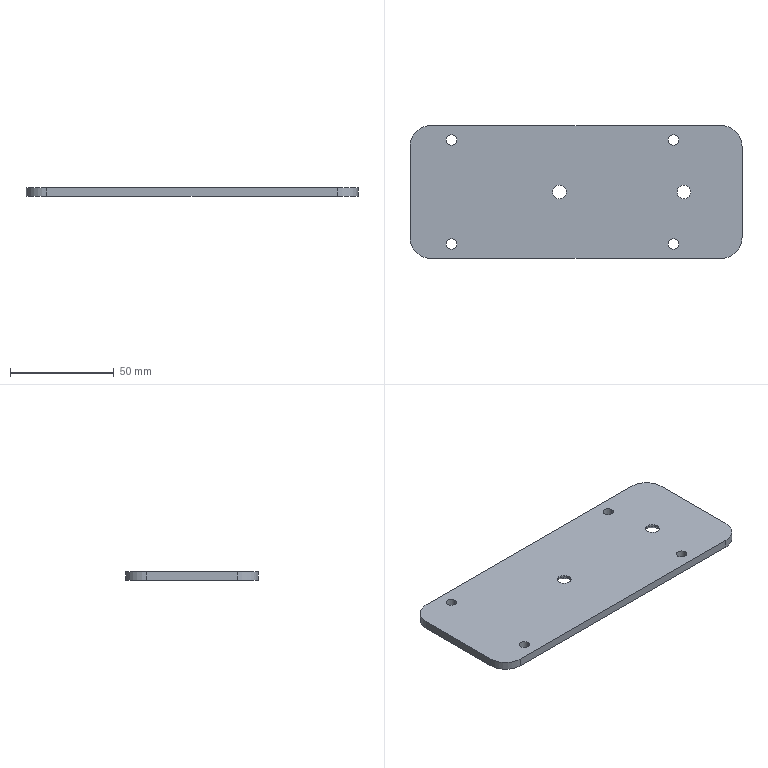Part | SolidWorks | features HoleWzd 2, Extrusion 1, Fillet 1 | 1 solid | 26 faces | box 160 x 64 x 4 mm | volume 39767 mm3 | cylinder 16 | plane 6 | cone 4 | commonest cylinder face diameters 5 x8 6.6 x4 20 x4
STEP:
#1=CARTESIAN_POINT('',(55.3,0.,3.1));
#2=VERTEX_POINT('',#1);
#3=CARTESIAN_POINT('',(48.7,0.,3.1));
#4=VERTEX_POINT('',#3);
#5=CARTESIAN_POINT('',(52.,0.,3.1));
#6=DIRECTION('',(0.,0.,-1.));
#7=DIRECTION('',(-1.,0.,0.));
#8=AXIS2_PLACEMENT_3D('',#5,#6,#7);
#9=CIRCLE('',#8,3.3);
#10=EDGE_CURVE('',#2,#4,#9,.T.);
#11=ORIENTED_EDGE('',*,*,#10,.F.);
#12=CARTESIAN_POINT('',(58.4,0.,0.));
#13=VERTEX_POINT('',#12);
#14=CARTESIAN_POINT('',(58.4,0.,0.));
#15=DIRECTION('',(0.7071,0.,-0.7071));
#16=VECTOR('',#15,1000.);
#17=LINE('',#14,#16);
#18=EDGE_CURVE('',#2,#13,#17,.T.);
#19=ORIENTED_EDGE('',*,*,#18,.T.);
#20=CARTESIAN_POINT('',(45.6,0.,0.));
#21=VERTEX_POINT('',#20);
#22=CARTESIAN_POINT('',(52.,0.,0.));
#23=DIRECTION('',(0.,0.,-1.));
#24=DIRECTION('',(-1.,0.,0.));
#25=AXIS2_PLACEMENT_3D('',#22,#23,#24);
#26=CIRCLE('',#25,6.4);
#27=EDGE_CURVE('',#13,#21,#26,.T.);
#28=ORIENTED_EDGE('',*,*,#27,.T.);
#29=CARTESIAN_POINT('',(45.6,0.,0.));
#30=DIRECTION('',(-0.7071,0.,-0.7071));
#31=VECTOR('',#30,1000.);
#32=LINE('',#29,#31);
#33=EDGE_CURVE('',#4,#21,#32,.T.);
#34=ORIENTED_EDGE('',*,*,#33,.F.);
#35=EDGE_LOOP('',(#11,#19,#28,#34));
#36=FACE_OUTER_BOUND('',#35,.T.);
#37=CARTESIAN_POINT('',(52.,0.,0.));
#38=DIRECTION('',(0.,0.,-1.));
#39=DIRECTION('',(-1.,0.,0.));
#40=AXIS2_PLACEMENT_3D('',#37,#38,#39);
#41=CONICAL_SURFACE('',#40,6.4,0.7854);
#42=ADVANCED_FACE('',(#36),#41,.F.);
#43=CARTESIAN_POINT('',(55.3,0.,4.));
#44=VERTEX_POINT('',#43);
#45=CARTESIAN_POINT('',(48.7,0.,4.));
#46=VERTEX_POINT('',#45);
#47=CARTESIAN_POINT('',(52.,0.,4.));
#48=DIRECTION('',(0.,0.,-1.));
#49=DIRECTION('',(-1.,0.,0.));
#50=AXIS2_PLACEMENT_3D('',#47,#48,#49);
#51=CIRCLE('',#50,3.3);
#52=EDGE_CURVE('',#44,#46,#51,.T.);
#53=ORIENTED_EDGE('',*,*,#52,.F.);
#54=CARTESIAN_POINT('',(55.3,0.,0.));
#55=DIRECTION('',(0.,0.,-1.));
#56=VECTOR('',#55,1000.);
#57=LINE('',#54,#56);
#58=EDGE_CURVE('',#44,#2,#57,.T.);
#59=ORIENTED_EDGE('',*,*,#58,.T.);
#60=ORIENTED_EDGE('',*,*,#10,.T.);
#61=CARTESIAN_POINT('',(48.7,0.,0.));
#62=DIRECTION('',(0.,0.,-1.));
#63=VECTOR('',#62,1000.);
#64=LINE('',#61,#63);
#65=EDGE_CURVE('',#46,#4,#64,.T.);
#66=ORIENTED_EDGE('',*,*,#65,.F.);
#67=EDGE_LOOP('',(#53,#59,#60,#66));
#68=FACE_OUTER_BOUND('',#67,.T.);
#69=CARTESIAN_POINT('',(52.,0.,0.));
#70=DIRECTION('',(0.,0.,-1.));
#71=DIRECTION('',(-1.,0.,0.));
#72=AXIS2_PLACEMENT_3D('',#69,#70,#71);
#73=CYLINDRICAL_SURFACE('',#72,3.3);
#74=ADVANCED_FACE('',(#68),#73,.F.);
#75=CARTESIAN_POINT('',(-4.7,0.,3.1));
#76=VERTEX_POINT('',#75);
#77=CARTESIAN_POINT('',(-11.3,0.,3.1));
#78=VERTEX_POINT('',#77);
#79=CARTESIAN_POINT('',(-8.,0.,3.1));
#80=DIRECTION('',(0.,0.,-1.));
#81=DIRECTION('',(-1.,0.,0.));
#82=AXIS2_PLACEMENT_3D('',#79,#80,#81);
#83=CIRCLE('',#82,3.3);
#84=EDGE_CURVE('',#76,#78,#83,.T.);
#85=ORIENTED_EDGE('',*,*,#84,.F.);
#86=CARTESIAN_POINT('',(-1.6,0.,0.));
#87=VERTEX_POINT('',#86);
#88=CARTESIAN_POINT('',(-1.6,0.,0.));
#89=DIRECTION('',(0.7071,0.,-0.7071));
#90=VECTOR('',#89,1000.);
#91=LINE('',#88,#90);
#92=EDGE_CURVE('',#76,#87,#91,.T.);
#93=ORIENTED_EDGE('',*,*,#92,.T.);
#94=CARTESIAN_POINT('',(-14.4,0.,0.));
#95=VERTEX_POINT('',#94);
#96=CARTESIAN_POINT('',(-8.,0.,0.));
#97=DIRECTION('',(0.,0.,-1.));
#98=DIRECTION('',(-1.,0.,0.));
#99=AXIS2_PLACEMENT_3D('',#96,#97,#98);
#100=CIRCLE('',#99,6.4);
#101=EDGE_CURVE('',#87,#95,#100,.T.);
#102=ORIENTED_EDGE('',*,*,#101,.T.);
#103=CARTESIAN_POINT('',(-14.4,0.,0.));
#104=DIRECTION('',(-0.7071,0.,-0.7071));
#105=VECTOR('',#104,1000.);
#106=LINE('',#103,#105);
#107=EDGE_CURVE('',#78,#95,#106,.T.);
#108=ORIENTED_EDGE('',*,*,#107,.F.);
#109=EDGE_LOOP('',(#85,#93,#102,#108));
#110=FACE_OUTER_BOUND('',#109,.T.);
#111=CARTESIAN_POINT('',(-8.,0.,0.));
#112=DIRECTION('',(0.,0.,-1.));
#113=DIRECTION('',(-1.,0.,0.));
#114=AXIS2_PLACEMENT_3D('',#111,#112,#113);
#115=CONICAL_SURFACE('',#114,6.4,0.7854);
#116=ADVANCED_FACE('',(#110),#115,.F.);
#117=CARTESIAN_POINT('',(-4.7,0.,4.));
#118=VERTEX_POINT('',#117);
#119=CARTESIAN_POINT('',(-11.3,0.,4.));
#120=VERTEX_POINT('',#119);
#121=CARTESIAN_POINT('',(-8.,0.,4.));
#122=DIRECTION('',(0.,0.,-1.));
#123=DIRECTION('',(-1.,0.,0.));
#124=AXIS2_PLACEMENT_3D('',#121,#122,#123);
#125=CIRCLE('',#124,3.3);
#126=EDGE_CURVE('',#118,#120,#125,.T.);
#127=ORIENTED_EDGE('',*,*,#126,.F.);
#128=CARTESIAN_POINT('',(-4.7,0.,0.));
#129=DIRECTION('',(0.,0.,-1.));
#130=VECTOR('',#129,1000.);
#131=LINE('',#128,#130);
#132=EDGE_CURVE('',#118,#76,#131,.T.);
#133=ORIENTED_EDGE('',*,*,#132,.T.);
#134=ORIENTED_EDGE('',*,*,#84,.T.);
#135=CARTESIAN_POINT('',(-11.3,0.,0.));
#136=DIRECTION('',(0.,0.,-1.));
#137=VECTOR('',#136,1000.);
#138=LINE('',#135,#137);
#139=EDGE_CURVE('',#120,#78,#138,.T.);
#140=ORIENTED_EDGE('',*,*,#139,.F.);
#141=EDGE_LOOP('',(#127,#133,#134,#140));
#142=FACE_OUTER_BOUND('',#141,.T.);
#143=CARTESIAN_POINT('',(-8.,0.,0.));
#144=DIRECTION('',(0.,0.,-1.));
#145=DIRECTION('',(-1.,0.,0.));
#146=AXIS2_PLACEMENT_3D('',#143,#144,#145);
#147=CYLINDRICAL_SURFACE('',#146,3.3);
#148=ADVANCED_FACE('',(#142),#147,.F.);
#149=CARTESIAN_POINT('',(-62.5,25.,0.));
#150=VERTEX_POINT('',#149);
#151=CARTESIAN_POINT('',(-57.5,25.,0.));
#152=VERTEX_POINT('',#151);
#153=CARTESIAN_POINT('',(-60.,25.,0.));
#154=DIRECTION('',(0.,0.,1.));
#155=DIRECTION('',(1.,0.,0.));
#156=AXIS2_PLACEMENT_3D('',#153,#154,#155);
#157=CIRCLE('',#156,2.5);
#158=EDGE_CURVE('',#150,#152,#157,.T.);
#159=ORIENTED_EDGE('',*,*,#158,.F.);
#160=CARTESIAN_POINT('',(-62.5,25.,4.));
#161=VERTEX_POINT('',#160);
#162=CARTESIAN_POINT('',(-62.5,25.,4.));
#163=DIRECTION('',(0.,0.,1.));
#164=VECTOR('',#163,1000.);
#165=LINE('',#162,#164);
#166=EDGE_CURVE('',#150,#161,#165,.T.);
#167=ORIENTED_EDGE('',*,*,#166,.T.);
#168=CARTESIAN_POINT('',(-57.5,25.,4.));
#169=VERTEX_POINT('',#168);
#170=CARTESIAN_POINT('',(-60.,25.,4.));
#171=DIRECTION('',(0.,0.,1.));
#172=DIRECTION('',(1.,0.,0.));
#173=AXIS2_PLACEMENT_3D('',#170,#171,#172);
#174=CIRCLE('',#173,2.5);
#175=EDGE_CURVE('',#161,#169,#174,.T.);
#176=ORIENTED_EDGE('',*,*,#175,.T.);
#177=CARTESIAN_POINT('',(-57.5,25.,4.));
#178=DIRECTION('',(0.,0.,1.));
#179=VECTOR('',#178,1000.);
#180=LINE('',#177,#179);
#181=EDGE_CURVE('',#152,#169,#180,.T.);
#182=ORIENTED_EDGE('',*,*,#181,.F.);
#183=EDGE_LOOP('',(#159,#167,#176,#182));
#184=FACE_OUTER_BOUND('',#183,.T.);
#185=CARTESIAN_POINT('',(-60.,25.,4.));
#186=DIRECTION('',(0.,0.,1.));
#187=DIRECTION('',(1.,0.,0.));
#188=AXIS2_PLACEMENT_3D('',#185,#186,#187);
#189=CYLINDRICAL_SURFACE('',#188,2.5);
#190=ADVANCED_FACE('',(#184),#189,.F.);
#191=CARTESIAN_POINT('',(-62.5,-25.,0.));
#192=VERTEX_POINT('',#191);
#193=CARTESIAN_POINT('',(-57.5,-25.,0.));
#194=VERTEX_POINT('',#193);
#195=CARTESIAN_POINT('',(-60.,-25.,0.));
#196=DIRECTION('',(0.,0.,1.));
#197=DIRECTION('',(1.,0.,0.));
#198=AXIS2_PLACEMENT_3D('',#195,#196,#197);
#199=CIRCLE('',#198,2.5);
#200=EDGE_CURVE('',#192,#194,#199,.T.);
#201=ORIENTED_EDGE('',*,*,#200,.F.);
#202=CARTESIAN_POINT('',(-62.5,-25.,4.));
#203=VERTEX_POINT('',#202);
#204=CARTESIAN_POINT('',(-62.5,-25.,4.));
#205=DIRECTION('',(0.,0.,1.));
#206=VECTOR('',#205,1000.);
#207=LINE('',#204,#206);
#208=EDGE_CURVE('',#192,#203,#207,.T.);
#209=ORIENTED_EDGE('',*,*,#208,.T.);
#210=CARTESIAN_POINT('',(-57.5,-25.,4.));
#211=VERTEX_POINT('',#210);
#212=CARTESIAN_POINT('',(-60.,-25.,4.));
#213=DIRECTION('',(0.,0.,1.));
#214=DIRECTION('',(1.,0.,0.));
#215=AXIS2_PLACEMENT_3D('',#212,#213,#214);
#216=CIRCLE('',#215,2.5);
#217=EDGE_CURVE('',#203,#211,#216,.T.);
#218=ORIENTED_EDGE('',*,*,#217,.T.);
#219=CARTESIAN_POINT('',(-57.5,-25.,4.));
#220=DIRECTION('',(0.,0.,1.));
#221=VECTOR('',#220,1000.);
#222=LINE('',#219,#221);
#223=EDGE_CURVE('',#194,#211,#222,.T.);
#224=ORIENTED_EDGE('',*,*,#223,.F.);
#225=EDGE_LOOP('',(#201,#209,#218,#224));
#226=FACE_OUTER_BOUND('',#225,.T.);
#227=CARTESIAN_POINT('',(-60.,-25.,4.));
#228=DIRECTION('',(0.,0.,1.));
#229=DIRECTION('',(1.,0.,0.));
#230=AXIS2_PLACEMENT_3D('',#227,#228,#229);
#231=CYLINDRICAL_SURFACE('',#230,2.5);
#232=ADVANCED_FACE('',(#226),#231,.F.);
#233=CARTESIAN_POINT('',(44.5,25.,0.));
#234=VERTEX_POINT('',#233);
#235=CARTESIAN_POINT('',(49.5,25.,0.));
#236=VERTEX_POINT('',#235);
#237=CARTESIAN_POINT('',(47.,25.,0.));
#238=DIRECTION('',(0.,0.,1.));
#239=DIRECTION('',(1.,0.,0.));
#240=AXIS2_PLACEMENT_3D('',#237,#238,#239);
#241=CIRCLE('',#240,2.5);
#242=EDGE_CURVE('',#234,#236,#241,.T.);
#243=ORIENTED_EDGE('',*,*,#242,.F.);
#244=CARTESIAN_POINT('',(44.5,25.,4.));
#245=VERTEX_POINT('',#244);
#246=CARTESIAN_POINT('',(44.5,25.,4.));
#247=DIRECTION('',(0.,0.,1.));
#248=VECTOR('',#247,1000.);
#249=LINE('',#246,#248);
#250=EDGE_CURVE('',#234,#245,#249,.T.);
#251=ORIENTED_EDGE('',*,*,#250,.T.);
#252=CARTESIAN_POINT('',(49.5,25.,4.));
#253=VERTEX_POINT('',#252);
#254=CARTESIAN_POINT('',(47.,25.,4.));
#255=DIRECTION('',(0.,0.,1.));
#256=DIRECTION('',(1.,0.,0.));
#257=AXIS2_PLACEMENT_3D('',#254,#255,#256);
#258=CIRCLE('',#257,2.5);
#259=EDGE_CURVE('',#245,#253,#258,.T.);
#260=ORIENTED_EDGE('',*,*,#259,.T.);
#261=CARTESIAN_POINT('',(49.5,25.,4.));
#262=DIRECTION('',(0.,0.,1.));
#263=VECTOR('',#262,1000.);
#264=LINE('',#261,#263);
#265=EDGE_CURVE('',#236,#253,#264,.T.);
#266=ORIENTED_EDGE('',*,*,#265,.F.);
#267=EDGE_LOOP('',(#243,#251,#260,#266));
#268=FACE_OUTER_BOUND('',#267,.T.);
#269=CARTESIAN_POINT('',(47.,25.,4.));
#270=DIRECTION('',(0.,0.,1.));
#271=DIRECTION('',(1.,0.,0.));
#272=AXIS2_PLACEMENT_3D('',#269,#270,#271);
#273=CYLINDRICAL_SURFACE('',#272,2.5);
#274=ADVANCED_FACE('',(#268),#273,.F.);
#275=CARTESIAN_POINT('',(44.5,-25.,0.));
#276=VERTEX_POINT('',#275);
#277=CARTESIAN_POINT('',(49.5,-25.,0.));
#278=VERTEX_POINT('',#277);
#279=CARTESIAN_POINT('',(47.,-25.,0.));
#280=DIRECTION('',(0.,0.,1.));
#281=DIRECTION('',(1.,0.,0.));
#282=AXIS2_PLACEMENT_3D('',#279,#280,#281);
#283=CIRCLE('',#282,2.5);
#284=EDGE_CURVE('',#276,#278,#283,.T.);
#285=ORIENTED_EDGE('',*,*,#284,.F.);
#286=CARTESIAN_POINT('',(44.5,-25.,4.));
#287=VERTEX_POINT('',#286);
#288=CARTESIAN_POINT('',(44.5,-25.,4.));
#289=DIRECTION('',(0.,0.,1.));
#290=VECTOR('',#289,1000.);
#291=LINE('',#288,#290);
#292=EDGE_CURVE('',#276,#287,#291,.T.);
#293=ORIENTED_EDGE('',*,*,#292,.T.);
#294=CARTESIAN_POINT('',(49.5,-25.,4.));
#295=VERTEX_POINT('',#294);
#296=CARTESIAN_POINT('',(47.,-25.,4.));
#297=DIRECTION('',(0.,0.,1.));
#298=DIRECTION('',(1.,0.,0.));
#299=AXIS2_PLACEMENT_3D('',#296,#297,#298);
#300=CIRCLE('',#299,2.5);
#301=EDGE_CURVE('',#287,#295,#300,.T.);
#302=ORIENTED_EDGE('',*,*,#301,.T.);
#303=CARTESIAN_POINT('',(49.5,-25.,4.));
#304=DIRECTION('',(0.,0.,1.));
#305=VECTOR('',#304,1000.);
#306=LINE('',#303,#305);
#307=EDGE_CURVE('',#278,#295,#306,.T.);
#308=ORIENTED_EDGE('',*,*,#307,.F.);
#309=EDGE_LOOP('',(#285,#293,#302,#308));
#310=FACE_OUTER_BOUND('',#309,.T.);
#311=CARTESIAN_POINT('',(47.,-25.,4.));
#312=DIRECTION('',(0.,0.,1.));
#313=DIRECTION('',(1.,0.,0.));
#314=AXIS2_PLACEMENT_3D('',#311,#312,#313);
#315=CYLINDRICAL_SURFACE('',#314,2.5);
#316=ADVANCED_FACE('',(#310),#315,.F.);
#317=CARTESIAN_POINT('',(80.,-22.,0.));
#318=VERTEX_POINT('',#317);
#319=CARTESIAN_POINT('',(80.,22.,0.));
#320=VERTEX_POINT('',#319);
#321=CARTESIAN_POINT('',(80.,32.,0.));
#322=DIRECTION('',(0.,1.,0.));
#323=VECTOR('',#322,1000.);
#324=LINE('',#321,#323);
#325=EDGE_CURVE('',#318,#320,#324,.T.);
#326=ORIENTED_EDGE('',*,*,#325,.T.);
#327=CARTESIAN_POINT('',(80.,22.,4.));
#328=VERTEX_POINT('',#327);
#329=CARTESIAN_POINT('',(80.,22.,4.));
#330=DIRECTION('',(0.,0.,1.));
#331=VECTOR('',#330,1000.);
#332=LINE('',#329,#331);
#333=EDGE_CURVE('',#320,#328,#332,.T.);
#334=ORIENTED_EDGE('',*,*,#333,.T.);
#335=CARTESIAN_POINT('',(80.,-22.,4.));
#336=VERTEX_POINT('',#335);
#337=CARTESIAN_POINT('',(80.,32.,4.));
#338=DIRECTION('',(0.,1.,0.));
#339=VECTOR('',#338,1000.);
#340=LINE('',#337,#339);
#341=EDGE_CURVE('',#336,#328,#340,.T.);
#342=ORIENTED_EDGE('',*,*,#341,.F.);
#343=CARTESIAN_POINT('',(80.,-22.,4.));
#344=DIRECTION('',(0.,0.,-1.));
#345=VECTOR('',#344,1000.);
#346=LINE('',#343,#345);
#347=EDGE_CURVE('',#336,#318,#346,.T.);
#348=ORIENTED_EDGE('',*,*,#347,.T.);
#349=EDGE_LOOP('',(#326,#334,#342,#348));
#350=FACE_OUTER_BOUND('',#349,.T.);
#351=CARTESIAN_POINT('',(80.,32.,4.));
#352=DIRECTION('',(-1.,0.,0.));
#353=DIRECTION('',(0.,0.,1.));
#354=AXIS2_PLACEMENT_3D('',#351,#352,#353);
#355=PLANE('',#354);
#356=ADVANCED_FACE('',(#350),#355,.F.);
#357=CARTESIAN_POINT('',(70.,32.,4.));
#358=VERTEX_POINT('',#357);
#359=CARTESIAN_POINT('',(-70.,32.,4.));
#360=VERTEX_POINT('',#359);
#361=CARTESIAN_POINT('',(-80.,32.,4.));
#362=DIRECTION('',(-1.,0.,0.));
#363=VECTOR('',#362,1000.);
#364=LINE('',#361,#363);
#365=EDGE_CURVE('',#358,#360,#364,.T.);
#366=ORIENTED_EDGE('',*,*,#365,.F.);
#367=CARTESIAN_POINT('',(70.,32.,0.));
#368=VERTEX_POINT('',#367);
#369=CARTESIAN_POINT('',(70.,32.,4.));
#370=DIRECTION('',(0.,0.,-1.));
#371=VECTOR('',#370,1000.);
#372=LINE('',#369,#371);
#373=EDGE_CURVE('',#358,#368,#372,.T.);
#374=ORIENTED_EDGE('',*,*,#373,.T.);
#375=CARTESIAN_POINT('',(-70.,32.,0.));
#376=VERTEX_POINT('',#375);
#377=CARTESIAN_POINT('',(-80.,32.,0.));
#378=DIRECTION('',(-1.,0.,0.));
#379=VECTOR('',#378,1000.);
#380=LINE('',#377,#379);
#381=EDGE_CURVE('',#368,#376,#380,.T.);
#382=ORIENTED_EDGE('',*,*,#381,.T.);
#383=CARTESIAN_POINT('',(-70.,32.,4.));
#384=DIRECTION('',(0.,0.,1.));
#385=VECTOR('',#384,1000.);
#386=LINE('',#383,#385);
#387=EDGE_CURVE('',#376,#360,#386,.T.);
#388=ORIENTED_EDGE('',*,*,#387,.T.);
#389=EDGE_LOOP('',(#366,#374,#382,#388));
#390=FACE_OUTER_BOUND('',#389,.T.);
#391=CARTESIAN_POINT('',(-80.,32.,4.));
#392=DIRECTION('',(0.,-1.,0.));
#393=DIRECTION('',(0.,0.,-1.));
#394=AXIS2_PLACEMENT_3D('',#391,#392,#393);
#395=PLANE('',#394);
#396=ADVANCED_FACE('',(#390),#395,.F.);
#397=CARTESIAN_POINT('',(-80.,22.,4.));
#398=VERTEX_POINT('',#397);
#399=CARTESIAN_POINT('',(-80.,-22.,4.));
#400=VERTEX_POINT('',#399);
#401=CARTESIAN_POINT('',(-80.,32.,4.));
#402=DIRECTION('',(0.,-1.,0.));
#403=VECTOR('',#402,1000.);
#404=LINE('',#401,#403);
#405=EDGE_CURVE('',#398,#400,#404,.T.);
#406=ORIENTED_EDGE('',*,*,#405,.F.);
#407=CARTESIAN_POINT('',(-80.,22.,0.));
#408=VERTEX_POINT('',#407);
#409=CARTESIAN_POINT('',(-80.,22.,4.));
#410=DIRECTION('',(0.,0.,-1.));
#411=VECTOR('',#410,1000.);
#412=LINE('',#409,#411);
#413=EDGE_CURVE('',#398,#408,#412,.T.);
#414=ORIENTED_EDGE('',*,*,#413,.T.);
#415=CARTESIAN_POINT('',(-80.,-22.,0.));
#416=VERTEX_POINT('',#415);
#417=CARTESIAN_POINT('',(-80.,32.,0.));
#418=DIRECTION('',(0.,-1.,0.));
#419=VECTOR('',#418,1000.);
#420=LINE('',#417,#419);
#421=EDGE_CURVE('',#408,#416,#420,.T.);
#422=ORIENTED_EDGE('',*,*,#421,.T.);
#423=CARTESIAN_POINT('',(-80.,-22.,4.));
#424=DIRECTION('',(0.,0.,1.));
#425=VECTOR('',#424,1000.);
#426=LINE('',#423,#425);
#427=EDGE_CURVE('',#416,#400,#426,.T.);
#428=ORIENTED_EDGE('',*,*,#427,.T.);
#429=EDGE_LOOP('',(#406,#414,#422,#428));
#430=FACE_OUTER_BOUND('',#429,.T.);
#431=CARTESIAN_POINT('',(-80.,32.,4.));
#432=DIRECTION('',(1.,0.,0.));
#433=DIRECTION('',(0.,1.,0.));
#434=AXIS2_PLACEMENT_3D('',#431,#432,#433);
#435=PLANE('',#434);
#436=ADVANCED_FACE('',(#430),#435,.F.);
#437=CARTESIAN_POINT('',(-70.,-32.,0.));
#438=VERTEX_POINT('',#437);
#439=CARTESIAN_POINT('',(70.,-32.,0.));
#440=VERTEX_POINT('',#439);
#441=CARTESIAN_POINT('',(-80.,-32.,0.));
#442=DIRECTION('',(1.,0.,0.));
#443=VECTOR('',#442,1000.);
#444=LINE('',#441,#443);
#445=EDGE_CURVE('',#438,#440,#444,.T.);
#446=ORIENTED_EDGE('',*,*,#445,.T.);
#447=CARTESIAN_POINT('',(70.,-32.,4.));
#448=VERTEX_POINT('',#447);
#449=CARTESIAN_POINT('',(70.,-32.,4.));
#450=DIRECTION('',(0.,0.,1.));
#451=VECTOR('',#450,1000.);
#452=LINE('',#449,#451);
#453=EDGE_CURVE('',#440,#448,#452,.T.);
#454=ORIENTED_EDGE('',*,*,#453,.T.);
#455=CARTESIAN_POINT('',(-70.,-32.,4.));
#456=VERTEX_POINT('',#455);
#457=CARTESIAN_POINT('',(-80.,-32.,4.));
#458=DIRECTION('',(1.,0.,0.));
#459=VECTOR('',#458,1000.);
#460=LINE('',#457,#459);
#461=EDGE_CURVE('',#456,#448,#460,.T.);
#462=ORIENTED_EDGE('',*,*,#461,.F.);
#463=CARTESIAN_POINT('',(-70.,-32.,4.));
#464=DIRECTION('',(0.,0.,-1.));
#465=VECTOR('',#464,1000.);
#466=LINE('',#463,#465);
#467=EDGE_CURVE('',#456,#438,#466,.T.);
#468=ORIENTED_EDGE('',*,*,#467,.T.);
#469=EDGE_LOOP('',(#446,#454,#462,#468));
#470=FACE_OUTER_BOUND('',#469,.T.);
#471=CARTESIAN_POINT('',(-80.,-32.,4.));
#472=DIRECTION('',(0.,1.,0.));
#473=DIRECTION('',(0.,0.,1.));
#474=AXIS2_PLACEMENT_3D('',#471,#472,#473);
#475=PLANE('',#474);
#476=ADVANCED_FACE('',(#470),#475,.F.);
#477=CARTESIAN_POINT('',(52.,0.,4.));
#478=DIRECTION('',(0.,0.,-1.));
#479=DIRECTION('',(-1.,0.,0.));
#480=AXIS2_PLACEMENT_3D('',#477,#478,#479);
#481=CIRCLE('',#480,3.3);
#482=EDGE_CURVE('',#46,#44,#481,.T.);
#483=ORIENTED_EDGE('',*,*,#482,.T.);
#484=ORIENTED_EDGE('',*,*,#52,.T.);
#485=EDGE_LOOP('',(#483,#484));
#486=FACE_BOUND('',#485,.T.);
#487=CARTESIAN_POINT('',(-8.,0.,4.));
#488=DIRECTION('',(0.,0.,-1.));
#489=DIRECTION('',(-1.,0.,0.));
#490=AXIS2_PLACEMENT_3D('',#487,#488,#489);
#491=CIRCLE('',#490,3.3);
#492=EDGE_CURVE('',#120,#118,#491,.T.);
#493=ORIENTED_EDGE('',*,*,#492,.T.);
#494=ORIENTED_EDGE('',*,*,#126,.T.);
#495=EDGE_LOOP('',(#493,#494));
#496=FACE_BOUND('',#495,.T.);
#497=CARTESIAN_POINT('',(-60.,25.,4.));
#498=DIRECTION('',(0.,0.,1.));
#499=DIRECTION('',(1.,0.,0.));
#500=AXIS2_PLACEMENT_3D('',#497,#498,#499);
#501=CIRCLE('',#500,2.5);
#502=EDGE_CURVE('',#169,#161,#501,.T.);
#503=ORIENTED_EDGE('',*,*,#502,.F.);
#504=ORIENTED_EDGE('',*,*,#175,.F.);
#505=EDGE_LOOP('',(#503,#504));
#506=FACE_BOUND('',#505,.T.);
#507=CARTESIAN_POINT('',(-60.,-25.,4.));
#508=DIRECTION('',(0.,0.,1.));
#509=DIRECTION('',(1.,0.,0.));
#510=AXIS2_PLACEMENT_3D('',#507,#508,#509);
#511=CIRCLE('',#510,2.5);
#512=EDGE_CURVE('',#211,#203,#511,.T.);
#513=ORIENTED_EDGE('',*,*,#512,.F.);
#514=ORIENTED_EDGE('',*,*,#217,.F.);
#515=EDGE_LOOP('',(#513,#514));
#516=FACE_BOUND('',#515,.T.);
#517=CARTESIAN_POINT('',(47.,25.,4.));
#518=DIRECTION('',(0.,0.,1.));
#519=DIRECTION('',(1.,0.,0.));
#520=AXIS2_PLACEMENT_3D('',#517,#518,#519);
#521=CIRCLE('',#520,2.5);
#522=EDGE_CURVE('',#253,#245,#521,.T.);
#523=ORIENTED_EDGE('',*,*,#522,.F.);
#524=ORIENTED_EDGE('',*,*,#259,.F.);
#525=EDGE_LOOP('',(#523,#524));
#526=FACE_BOUND('',#525,.T.);
#527=CARTESIAN_POINT('',(47.,-25.,4.));
#528=DIRECTION('',(0.,0.,1.));
#529=DIRECTION('',(1.,0.,0.));
#530=AXIS2_PLACEMENT_3D('',#527,#528,#529);
#531=CIRCLE('',#530,2.5);
#532=EDGE_CURVE('',#295,#287,#531,.T.);
#533=ORIENTED_EDGE('',*,*,#532,.F.);
#534=ORIENTED_EDGE('',*,*,#301,.F.);
#535=EDGE_LOOP('',(#533,#534));
#536=FACE_BOUND('',#535,.T.);
#537=ORIENTED_EDGE('',*,*,#341,.T.);
#538=CARTESIAN_POINT('',(70.,22.,4.));
#539=DIRECTION('',(0.,0.,1.));
#540=DIRECTION('',(1.,0.,0.));
#541=AXIS2_PLACEMENT_3D('',#538,#539,#540);
#542=CIRCLE('',#541,10.);
#543=EDGE_CURVE('',#328,#358,#542,.T.);
#544=ORIENTED_EDGE('',*,*,#543,.T.);
#545=ORIENTED_EDGE('',*,*,#365,.T.);
#546=CARTESIAN_POINT('',(-70.,22.,4.));
#547=DIRECTION('',(0.,0.,1.));
#548=DIRECTION('',(1.,0.,0.));
#549=AXIS2_PLACEMENT_3D('',#546,#547,#548);
#550=CIRCLE('',#549,10.);
#551=EDGE_CURVE('',#360,#398,#550,.T.);
#552=ORIENTED_EDGE('',*,*,#551,.T.);
#553=ORIENTED_EDGE('',*,*,#405,.T.);
#554=CARTESIAN_POINT('',(-70.,-22.,4.));
#555=DIRECTION('',(0.,0.,1.));
#556=DIRECTION('',(1.,0.,0.));
#557=AXIS2_PLACEMENT_3D('',#554,#555,#556);
#558=CIRCLE('',#557,10.);
#559=EDGE_CURVE('',#400,#456,#558,.T.);
#560=ORIENTED_EDGE('',*,*,#559,.T.);
#561=ORIENTED_EDGE('',*,*,#461,.T.);
#562=CARTESIAN_POINT('',(70.,-22.,4.));
#563=DIRECTION('',(0.,0.,1.));
#564=DIRECTION('',(1.,0.,0.));
#565=AXIS2_PLACEMENT_3D('',#562,#563,#564);
#566=CIRCLE('',#565,10.);
#567=EDGE_CURVE('',#448,#336,#566,.T.);
#568=ORIENTED_EDGE('',*,*,#567,.T.);
#569=EDGE_LOOP('',(#537,#544,#545,#552,#553,#560,#561,#568));
#570=FACE_OUTER_BOUND('',#569,.T.);
#571=CARTESIAN_POINT('',(0.,0.,4.));
#572=DIRECTION('',(0.,0.,1.));
#573=DIRECTION('',(1.,0.,0.));
#574=AXIS2_PLACEMENT_3D('',#571,#572,#573);
#575=PLANE('',#574);
#576=ADVANCED_FACE('',(#486,#496,#506,#516,#526,#536,#570),#575,.T.);
#577=CARTESIAN_POINT('',(52.,0.,0.));
#578=DIRECTION('',(0.,0.,-1.));
#579=DIRECTION('',(-1.,0.,0.));
#580=AXIS2_PLACEMENT_3D('',#577,#578,#579);
#581=CIRCLE('',#580,6.4);
#582=EDGE_CURVE('',#21,#13,#581,.T.);
#583=ORIENTED_EDGE('',*,*,#582,.F.);
#584=ORIENTED_EDGE('',*,*,#27,.F.);
#585=EDGE_LOOP('',(#583,#584));
#586=FACE_BOUND('',#585,.T.);
#587=CARTESIAN_POINT('',(-8.,0.,0.));
#588=DIRECTION('',(0.,0.,-1.));
#589=DIRECTION('',(-1.,0.,0.));
#590=AXIS2_PLACEMENT_3D('',#587,#588,#589);
#591=CIRCLE('',#590,6.4);
#592=EDGE_CURVE('',#95,#87,#591,.T.);
#593=ORIENTED_EDGE('',*,*,#592,.F.);
#594=ORIENTED_EDGE('',*,*,#101,.F.);
#595=EDGE_LOOP('',(#593,#594));
#596=FACE_BOUND('',#595,.T.);
#597=CARTESIAN_POINT('',(-60.,25.,0.));
#598=DIRECTION('',(0.,0.,1.));
#599=DIRECTION('',(1.,0.,0.));
#600=AXIS2_PLACEMENT_3D('',#597,#598,#599);
#601=CIRCLE('',#600,2.5);
#602=EDGE_CURVE('',#152,#150,#601,.T.);
#603=ORIENTED_EDGE('',*,*,#602,.T.);
#604=ORIENTED_EDGE('',*,*,#158,.T.);
#605=EDGE_LOOP('',(#603,#604));
#606=FACE_BOUND('',#605,.T.);
#607=CARTESIAN_POINT('',(-60.,-25.,0.));
#608=DIRECTION('',(0.,0.,1.));
#609=DIRECTION('',(1.,0.,0.));
#610=AXIS2_PLACEMENT_3D('',#607,#608,#609);
#611=CIRCLE('',#610,2.5);
#612=EDGE_CURVE('',#194,#192,#611,.T.);
#613=ORIENTED_EDGE('',*,*,#612,.T.);
#614=ORIENTED_EDGE('',*,*,#200,.T.);
#615=EDGE_LOOP('',(#613,#614));
#616=FACE_BOUND('',#615,.T.);
#617=CARTESIAN_POINT('',(47.,25.,0.));
#618=DIRECTION('',(0.,0.,1.));
#619=DIRECTION('',(1.,0.,0.));
#620=AXIS2_PLACEMENT_3D('',#617,#618,#619);
#621=CIRCLE('',#620,2.5);
#622=EDGE_CURVE('',#236,#234,#621,.T.);
#623=ORIENTED_EDGE('',*,*,#622,.T.);
#624=ORIENTED_EDGE('',*,*,#242,.T.);
#625=EDGE_LOOP('',(#623,#624));
#626=FACE_BOUND('',#625,.T.);
#627=CARTESIAN_POINT('',(47.,-25.,0.));
#628=DIRECTION('',(0.,0.,1.));
#629=DIRECTION('',(1.,0.,0.));
#630=AXIS2_PLACEMENT_3D('',#627,#628,#629);
#631=CIRCLE('',#630,2.5);
#632=EDGE_CURVE('',#278,#276,#631,.T.);
#633=ORIENTED_EDGE('',*,*,#632,.T.);
#634=ORIENTED_EDGE('',*,*,#284,.T.);
#635=EDGE_LOOP('',(#633,#634));
#636=FACE_BOUND('',#635,.T.);
#637=ORIENTED_EDGE('',*,*,#381,.F.);
#638=CARTESIAN_POINT('',(70.,22.,0.));
#639=DIRECTION('',(0.,0.,-1.));
#640=DIRECTION('',(1.,0.,0.));
#641=AXIS2_PLACEMENT_3D('',#638,#639,#640);
#642=CIRCLE('',#641,10.);
#643=EDGE_CURVE('',#368,#320,#642,.T.);
#644=ORIENTED_EDGE('',*,*,#643,.T.);
#645=ORIENTED_EDGE('',*,*,#325,.F.);
#646=CARTESIAN_POINT('',(70.,-22.,0.));
#647=DIRECTION('',(0.,0.,-1.));
#648=DIRECTION('',(1.,0.,0.));
#649=AXIS2_PLACEMENT_3D('',#646,#647,#648);
#650=CIRCLE('',#649,10.);
#651=EDGE_CURVE('',#318,#440,#650,.T.);
#652=ORIENTED_EDGE('',*,*,#651,.T.);
#653=ORIENTED_EDGE('',*,*,#445,.F.);
#654=CARTESIAN_POINT('',(-70.,-22.,0.));
#655=DIRECTION('',(0.,0.,-1.));
#656=DIRECTION('',(1.,0.,0.));
#657=AXIS2_PLACEMENT_3D('',#654,#655,#656);
#658=CIRCLE('',#657,10.);
#659=EDGE_CURVE('',#438,#416,#658,.T.);
#660=ORIENTED_EDGE('',*,*,#659,.T.);
#661=ORIENTED_EDGE('',*,*,#421,.F.);
#662=CARTESIAN_POINT('',(-70.,22.,0.));
#663=DIRECTION('',(0.,0.,-1.));
#664=DIRECTION('',(1.,0.,0.));
#665=AXIS2_PLACEMENT_3D('',#662,#663,#664);
#666=CIRCLE('',#665,10.);
#667=EDGE_CURVE('',#408,#376,#666,.T.);
#668=ORIENTED_EDGE('',*,*,#667,.T.);
#669=EDGE_LOOP('',(#637,#644,#645,#652,#653,#660,#661,#668));
#670=FACE_OUTER_BOUND('',#669,.T.);
#671=CARTESIAN_POINT('',(0.,0.,0.));
#672=DIRECTION('',(0.,0.,1.));
#673=DIRECTION('',(1.,0.,0.));
#674=AXIS2_PLACEMENT_3D('',#671,#672,#673);
#675=PLANE('',#674);
#676=ADVANCED_FACE('',(#586,#596,#606,#616,#626,#636,#670),#675,.F.);
#677=ORIENTED_EDGE('',*,*,#543,.F.);
#678=ORIENTED_EDGE('',*,*,#333,.F.);
#679=ORIENTED_EDGE('',*,*,#643,.F.);
#680=ORIENTED_EDGE('',*,*,#373,.F.);
#681=EDGE_LOOP('',(#677,#678,#679,#680));
#682=FACE_OUTER_BOUND('',#681,.T.);
#683=CARTESIAN_POINT('',(70.,22.,4.));
#684=DIRECTION('',(0.,0.,-1.));
#685=DIRECTION('',(-1.,0.,0.));
#686=AXIS2_PLACEMENT_3D('',#683,#684,#685);
#687=CYLINDRICAL_SURFACE('',#686,10.);
#688=ADVANCED_FACE('',(#682),#687,.T.);
#689=ORIENTED_EDGE('',*,*,#567,.F.);
#690=ORIENTED_EDGE('',*,*,#453,.F.);
#691=ORIENTED_EDGE('',*,*,#651,.F.);
#692=ORIENTED_EDGE('',*,*,#347,.F.);
#693=EDGE_LOOP('',(#689,#690,#691,#692));
#694=FACE_OUTER_BOUND('',#693,.T.);
#695=CARTESIAN_POINT('',(70.,-22.,4.));
#696=DIRECTION('',(0.,0.,-1.));
#697=DIRECTION('',(-1.,0.,0.));
#698=AXIS2_PLACEMENT_3D('',#695,#696,#697);
#699=CYLINDRICAL_SURFACE('',#698,10.);
#700=ADVANCED_FACE('',(#694),#699,.T.);
#701=ORIENTED_EDGE('',*,*,#551,.F.);
#702=ORIENTED_EDGE('',*,*,#387,.F.);
#703=ORIENTED_EDGE('',*,*,#667,.F.);
#704=ORIENTED_EDGE('',*,*,#413,.F.);
#705=EDGE_LOOP('',(#701,#702,#703,#704));
#706=FACE_OUTER_BOUND('',#705,.T.);
#707=CARTESIAN_POINT('',(-70.,22.,4.));
#708=DIRECTION('',(0.,0.,-1.));
#709=DIRECTION('',(-1.,0.,0.));
#710=AXIS2_PLACEMENT_3D('',#707,#708,#709);
#711=CYLINDRICAL_SURFACE('',#710,10.);
#712=ADVANCED_FACE('',(#706),#711,.T.);
#713=ORIENTED_EDGE('',*,*,#559,.F.);
#714=ORIENTED_EDGE('',*,*,#427,.F.);
#715=ORIENTED_EDGE('',*,*,#659,.F.);
#716=ORIENTED_EDGE('',*,*,#467,.F.);
#717=EDGE_LOOP('',(#713,#714,#715,#716));
#718=FACE_OUTER_BOUND('',#717,.T.);
#719=CARTESIAN_POINT('',(-70.,-22.,4.));
#720=DIRECTION('',(0.,0.,-1.));
#721=DIRECTION('',(-1.,0.,0.));
#722=AXIS2_PLACEMENT_3D('',#719,#720,#721);
#723=CYLINDRICAL_SURFACE('',#722,10.);
#724=ADVANCED_FACE('',(#718),#723,.T.);
#725=ORIENTED_EDGE('',*,*,#292,.F.);
#726=ORIENTED_EDGE('',*,*,#632,.F.);
#727=ORIENTED_EDGE('',*,*,#307,.T.);
#728=ORIENTED_EDGE('',*,*,#532,.T.);
#729=EDGE_LOOP('',(#725,#726,#727,#728));
#730=FACE_OUTER_BOUND('',#729,.T.);
#731=CARTESIAN_POINT('',(47.,-25.,4.));
#732=DIRECTION('',(0.,0.,1.));
#733=DIRECTION('',(1.,0.,0.));
#734=AXIS2_PLACEMENT_3D('',#731,#732,#733);
#735=CYLINDRICAL_SURFACE('',#734,2.5);
#736=ADVANCED_FACE('',(#730),#735,.F.);
#737=ORIENTED_EDGE('',*,*,#250,.F.);
#738=ORIENTED_EDGE('',*,*,#622,.F.);
#739=ORIENTED_EDGE('',*,*,#265,.T.);
#740=ORIENTED_EDGE('',*,*,#522,.T.);
#741=EDGE_LOOP('',(#737,#738,#739,#740));
#742=FACE_OUTER_BOUND('',#741,.T.);
#743=CARTESIAN_POINT('',(47.,25.,4.));
#744=DIRECTION('',(0.,0.,1.));
#745=DIRECTION('',(1.,0.,0.));
#746=AXIS2_PLACEMENT_3D('',#743,#744,#745);
#747=CYLINDRICAL_SURFACE('',#746,2.5);
#748=ADVANCED_FACE('',(#742),#747,.F.);
#749=ORIENTED_EDGE('',*,*,#208,.F.);
#750=ORIENTED_EDGE('',*,*,#612,.F.);
#751=ORIENTED_EDGE('',*,*,#223,.T.);
#752=ORIENTED_EDGE('',*,*,#512,.T.);
#753=EDGE_LOOP('',(#749,#750,#751,#752));
#754=FACE_OUTER_BOUND('',#753,.T.);
#755=CARTESIAN_POINT('',(-60.,-25.,4.));
#756=DIRECTION('',(0.,0.,1.));
#757=DIRECTION('',(1.,0.,0.));
#758=AXIS2_PLACEMENT_3D('',#755,#756,#757);
#759=CYLINDRICAL_SURFACE('',#758,2.5);
#760=ADVANCED_FACE('',(#754),#759,.F.);
#761=ORIENTED_EDGE('',*,*,#166,.F.);
#762=ORIENTED_EDGE('',*,*,#602,.F.);
#763=ORIENTED_EDGE('',*,*,#181,.T.);
#764=ORIENTED_EDGE('',*,*,#502,.T.);
#765=EDGE_LOOP('',(#761,#762,#763,#764));
#766=FACE_OUTER_BOUND('',#765,.T.);
#767=CARTESIAN_POINT('',(-60.,25.,4.));
#768=DIRECTION('',(0.,0.,1.));
#769=DIRECTION('',(1.,0.,0.));
#770=AXIS2_PLACEMENT_3D('',#767,#768,#769);
#771=CYLINDRICAL_SURFACE('',#770,2.5);
#772=ADVANCED_FACE('',(#766),#771,.F.);
#773=ORIENTED_EDGE('',*,*,#132,.F.);
#774=ORIENTED_EDGE('',*,*,#492,.F.);
#775=ORIENTED_EDGE('',*,*,#139,.T.);
#776=CARTESIAN_POINT('',(-8.,0.,3.1));
#777=DIRECTION('',(0.,0.,-1.));
#778=DIRECTION('',(-1.,0.,0.));
#779=AXIS2_PLACEMENT_3D('',#776,#777,#778);
#780=CIRCLE('',#779,3.3);
#781=EDGE_CURVE('',#78,#76,#780,.T.);
#782=ORIENTED_EDGE('',*,*,#781,.T.);
#783=EDGE_LOOP('',(#773,#774,#775,#782));
#784=FACE_OUTER_BOUND('',#783,.T.);
#785=CARTESIAN_POINT('',(-8.,0.,0.));
#786=DIRECTION('',(0.,0.,-1.));
#787=DIRECTION('',(-1.,0.,0.));
#788=AXIS2_PLACEMENT_3D('',#785,#786,#787);
#789=CYLINDRICAL_SURFACE('',#788,3.3);
#790=ADVANCED_FACE('',(#784),#789,.F.);
#791=ORIENTED_EDGE('',*,*,#92,.F.);
#792=ORIENTED_EDGE('',*,*,#781,.F.);
#793=ORIENTED_EDGE('',*,*,#107,.T.);
#794=ORIENTED_EDGE('',*,*,#592,.T.);
#795=EDGE_LOOP('',(#791,#792,#793,#794));
#796=FACE_OUTER_BOUND('',#795,.T.);
#797=CARTESIAN_POINT('',(-8.,0.,0.));
#798=DIRECTION('',(0.,0.,-1.));
#799=DIRECTION('',(-1.,0.,0.));
#800=AXIS2_PLACEMENT_3D('',#797,#798,#799);
#801=CONICAL_SURFACE('',#800,6.4,0.7854);
#802=ADVANCED_FACE('',(#796),#801,.F.);
#803=ORIENTED_EDGE('',*,*,#58,.F.);
#804=ORIENTED_EDGE('',*,*,#482,.F.);
#805=ORIENTED_EDGE('',*,*,#65,.T.);
#806=CARTESIAN_POINT('',(52.,0.,3.1));
#807=DIRECTION('',(0.,0.,-1.));
#808=DIRECTION('',(-1.,0.,0.));
#809=AXIS2_PLACEMENT_3D('',#806,#807,#808);
#810=CIRCLE('',#809,3.3);
#811=EDGE_CURVE('',#4,#2,#810,.T.);
#812=ORIENTED_EDGE('',*,*,#811,.T.);
#813=EDGE_LOOP('',(#803,#804,#805,#812));
#814=FACE_OUTER_BOUND('',#813,.T.);
#815=CARTESIAN_POINT('',(52.,0.,0.));
#816=DIRECTION('',(0.,0.,-1.));
#817=DIRECTION('',(-1.,0.,0.));
#818=AXIS2_PLACEMENT_3D('',#815,#816,#817);
#819=CYLINDRICAL_SURFACE('',#818,3.3);
#820=ADVANCED_FACE('',(#814),#819,.F.);
#821=ORIENTED_EDGE('',*,*,#18,.F.);
#822=ORIENTED_EDGE('',*,*,#811,.F.);
#823=ORIENTED_EDGE('',*,*,#33,.T.);
#824=ORIENTED_EDGE('',*,*,#582,.T.);
#825=EDGE_LOOP('',(#821,#822,#823,#824));
#826=FACE_OUTER_BOUND('',#825,.T.);
#827=CARTESIAN_POINT('',(52.,0.,0.));
#828=DIRECTION('',(0.,0.,-1.));
#829=DIRECTION('',(-1.,0.,0.));
#830=AXIS2_PLACEMENT_3D('',#827,#828,#829);
#831=CONICAL_SURFACE('',#830,6.4,0.7854);
#832=ADVANCED_FACE('',(#826),#831,.F.);
#833=CLOSED_SHELL('',(#42,#74,#116,#148,#190,#232,#274,#316,#356,#396,#436,#476,#576,#676,#688,#700,#712,#724,#736,#748,#760,#772,#790,#802,#820,#832));
#834=MANIFOLD_SOLID_BREP('',#833);
#835=CARTESIAN_POINT('',(0.,0.,0.));
#836=DIRECTION('',(0.,0.,1.));
#837=DIRECTION('',(1.,0.,0.));
#838=AXIS2_PLACEMENT_3D('',#835,#836,#837);
#839=(LENGTH_UNIT()NAMED_UNIT(*)SI_UNIT(.MILLI.,.METRE.));
#840=UNCERTAINTY_MEASURE_WITH_UNIT(LENGTH_MEASURE(0.00001),#839,'','');
#841=(NAMED_UNIT(*)PLANE_ANGLE_UNIT()SI_UNIT($,.RADIAN.));
#842=(NAMED_UNIT(*)SI_UNIT($,.STERADIAN.)SOLID_ANGLE_UNIT());
#843=(GEOMETRIC_REPRESENTATION_CONTEXT(3)GLOBAL_UNCERTAINTY_ASSIGNED_CONTEXT((#840))GLOBAL_UNIT_ASSIGNED_CONTEXT((#839,#841,#842))REPRESENTATION_CONTEXT('',''));
#844=ADVANCED_BREP_SHAPE_REPRESENTATION('',(#834,#838),#843);